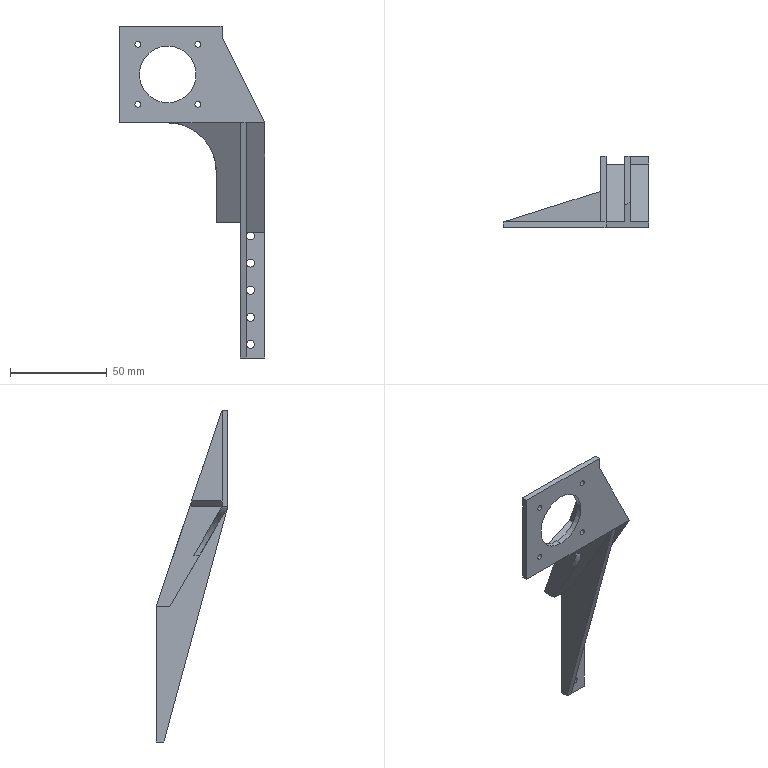Part | STEP file | Rear stepper bracket | 1 solid | 51 faces | box 75 x 37 x 171.474 mm | volume 24600 mm3 | plane 30 | cylinder 21 | commonest cylinder face diameters 4.1 x10 3 x8 29.321 x2 50 x1